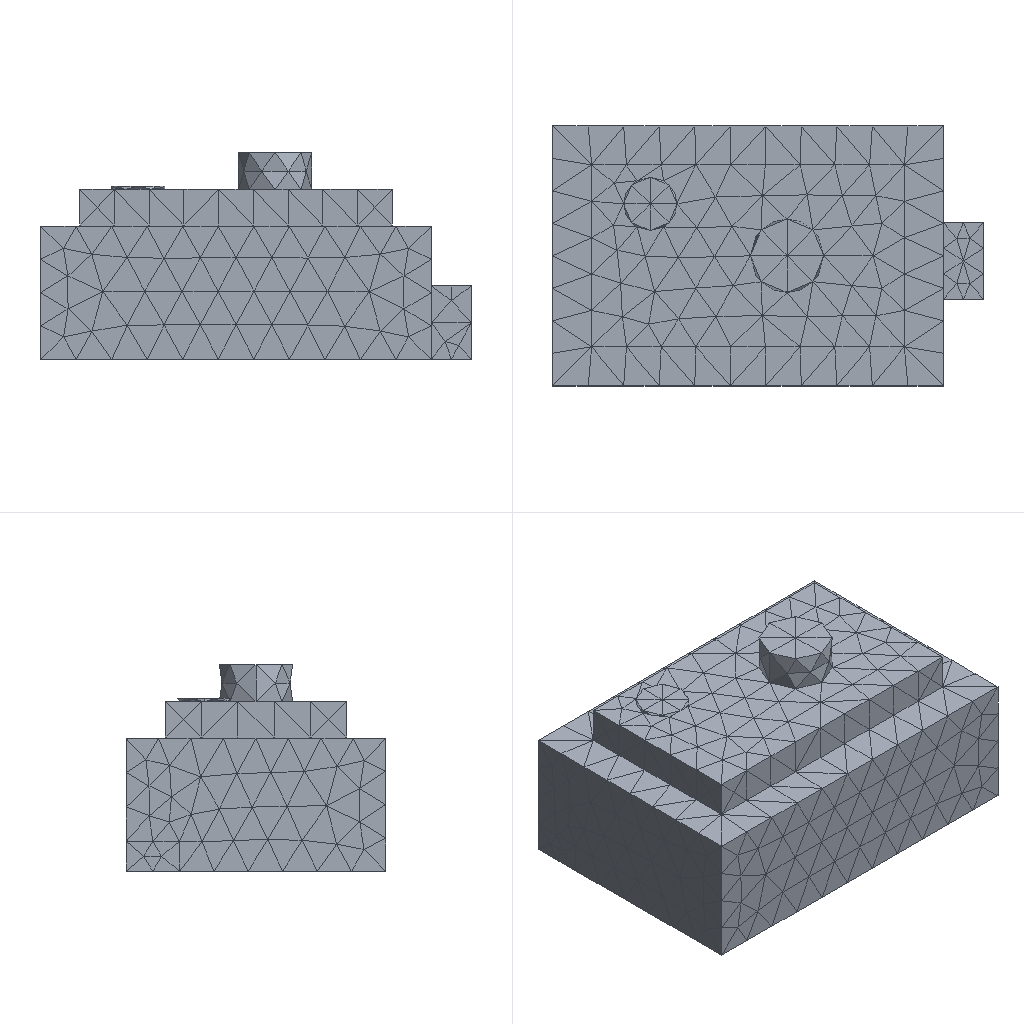Simulation study | ansys mapdl
Set-up summary:
category,name,step,type,value,unit,region
solver,ansys_mapdl
units,mm-N-s-tonne (MPa),,inferred,E=210000 density=
analysis,model,,static
mesh,nodes,,,5619
mesh,elements,,,3439
element_type,SOLID187,,,3439
material,mat 1,,E,210000
material,mat 1,,nu,0.3
load,,model,body load temp,,,all
load,,model,force,"1000 [dir=(0, 0, -1) n=416]",,node list
bc,,model,fixed,"[dofs=UX,UY,UZ n=6248]",,node list
Ansys APDL input file, long lists of numbers shortened:
/COM,ANSYS RELEASE 2026 R1           BUILD 26.1      UP20260202       09:11:27
/PREP7
/NOPR
/TITLE,2
ANTYPE, 0
*IF,_CDRDOFF,EQ,1,THEN     !if solid model was read in
_CDRDOFF=             !reset flag, numoffs already performed
*ELSE              !offset database for the following FE model
NUMOFF,NODE,     5619
NUMOFF,ELEM,     3439
NUMOFF,MAT ,        1
NUMOFF,TYPE,        1
*ENDIF
*SET,_RETURN ,  0.
*SET,_STATUS ,  0.
*SET,_UIQR   ,  416.
*SET,__FLOATPARAMETER__,  5619.
DOF,DELETE
ETBLOCK,        1,        1
(2i9,19a9)
        1      187        0        0        0        0        0        0        0        0        0        0        0        0        0        0        0        0        0        0        0
       -1
NBLOCK,6,SOLID,      5619,      5619
(3i9,6e21.13e3)
        1        0        0-4.2650000000000E+001 3.9000000000000E+001 9.0000000000000E+000
! (5618 more lines like these left out)
N,UNBL,LOC,       -1,
EBLOCK,19,SOLID,      3439,      3439
(19i10)
         1         1         1         1         0         0         0         0        10         0         1      1590      1598      1959      1599      1555      2314      2315      1554
! (6877 more lines like these left out)
        -1
MPTEMP,UNBL, 1, 1,  0.    ,
MPDATA,UNBL, 1,EX  ,       1, 1,  210000.000    ,
MPTEMP,UNBL, 1, 1,  0.    ,
MPDATA,UNBL, 1,NUXY,       1, 1, 0.3    ,
MPTEMP,UNBL, 1, 1,  0.    ,
MPDATA,UNBL, 1,PRXY,       1, 1, 0.3    ,
EXTOPT,ATTR,      0,      0,      0
EXTOPT,ESIZE,  0,  0.
EXTOPT,ACLEAR,      0
TREF,  0.
IRLF,  0
BFUNIF,TEMP,_TINY
ACEL,  0.    ,  0.    ,  0.
OMEGA,  0.    ,  0.    ,  0.
DOMEGA,  0.    ,  0.    ,  0.
CGLOC,  0.    ,  0.    ,  0.
CGOMEGA,  0.    ,  0.    ,  0.
DCGOMG,  0.    ,  0.    ,  0.
KUSE,     0
TIME,  0.
ALPHAD,  0.
BETAD,  0.
DMPRAT,  0.
DMPSTR,  0.
CRPLIM, 0.1    ,   0
CRPLIM,  0.    ,   1
NCNV,     0, 1.000000000E+12,     0,  0.    ,  0.
NEQIT,     0
ERESX,DEFA
DBLOCK,      6248
(i9,a6,2(pg16.9))
        1  UX    0.00000000      0.00000000
! (6247 more lines like these left out)
       -1
FBLOCK,       416
(i9,a6,2(pg16.9))
      611  FZ   -2.40384615      0.00000000
! (415 more lines like these left out)
       -1
/GO
FINISH
Results summary:
result,analysis_type_db,,,static,unstated
result,n_sets,,,1,unstated
result,load_steps[0].set,load_step=1,,1,unstated
result,load_steps[0].substep,load_step=1,,1,unstated
result,load_steps[0].time,load_step=1,,1,unstated
result,load_steps[0].freq,load_step=1,,1,unstated
result,load_steps[0].max_usum,load_step=1,,8.7232e-05,unstated
result,load_steps[0].max_seqv,load_step=1,,9.914,unstated
result,load_steps[0].reaction_sum.FX,load_step=1,,-3.2887e-12,unstated
result,load_steps[0].reaction_sum.FY,load_step=1,,-1.69914e-11,unstated
result,load_steps[0].reaction_sum.FZ,load_step=1,,1000,unstated
result,load_steps[0].reaction_sum.MX,load_step=1,,0,unstated
result,load_steps[0].reaction_sum.MY,load_step=1,,0,unstated
result,load_steps[0].reaction_sum.MZ,load_step=1,,0,unstated
result,convergence,,,results present for all listed sets,unstated